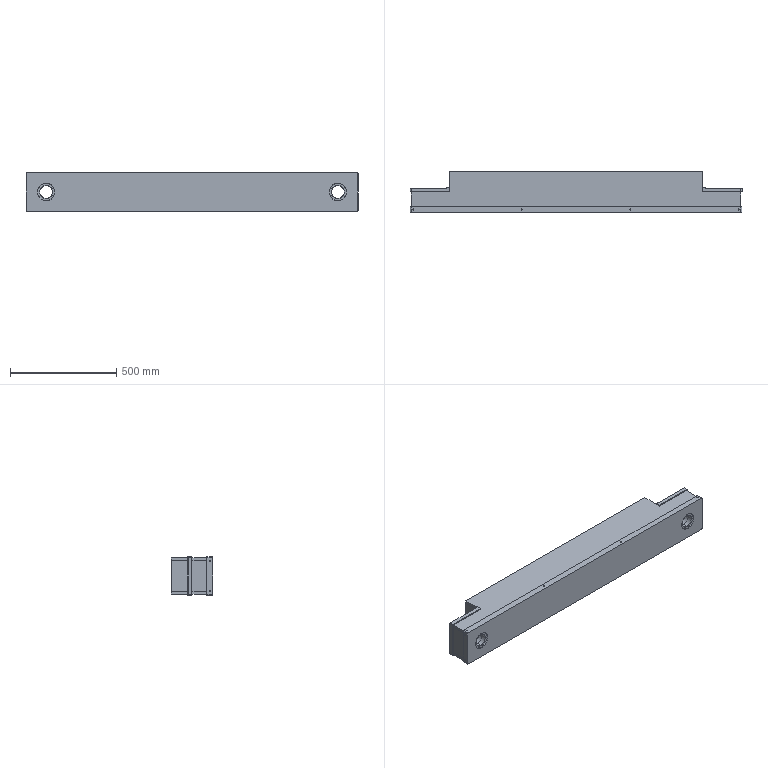Part | SolidWorks | 18 solids | 236 faces | box 1560 x 195 x 180 mm | volume 18777995 mm3 | plane 132 | cylinder 60 | cone 44 | commonest cylinder face diameters 5 x24 10 x8 10.2 x8 60 x8 80 x4 100 x4